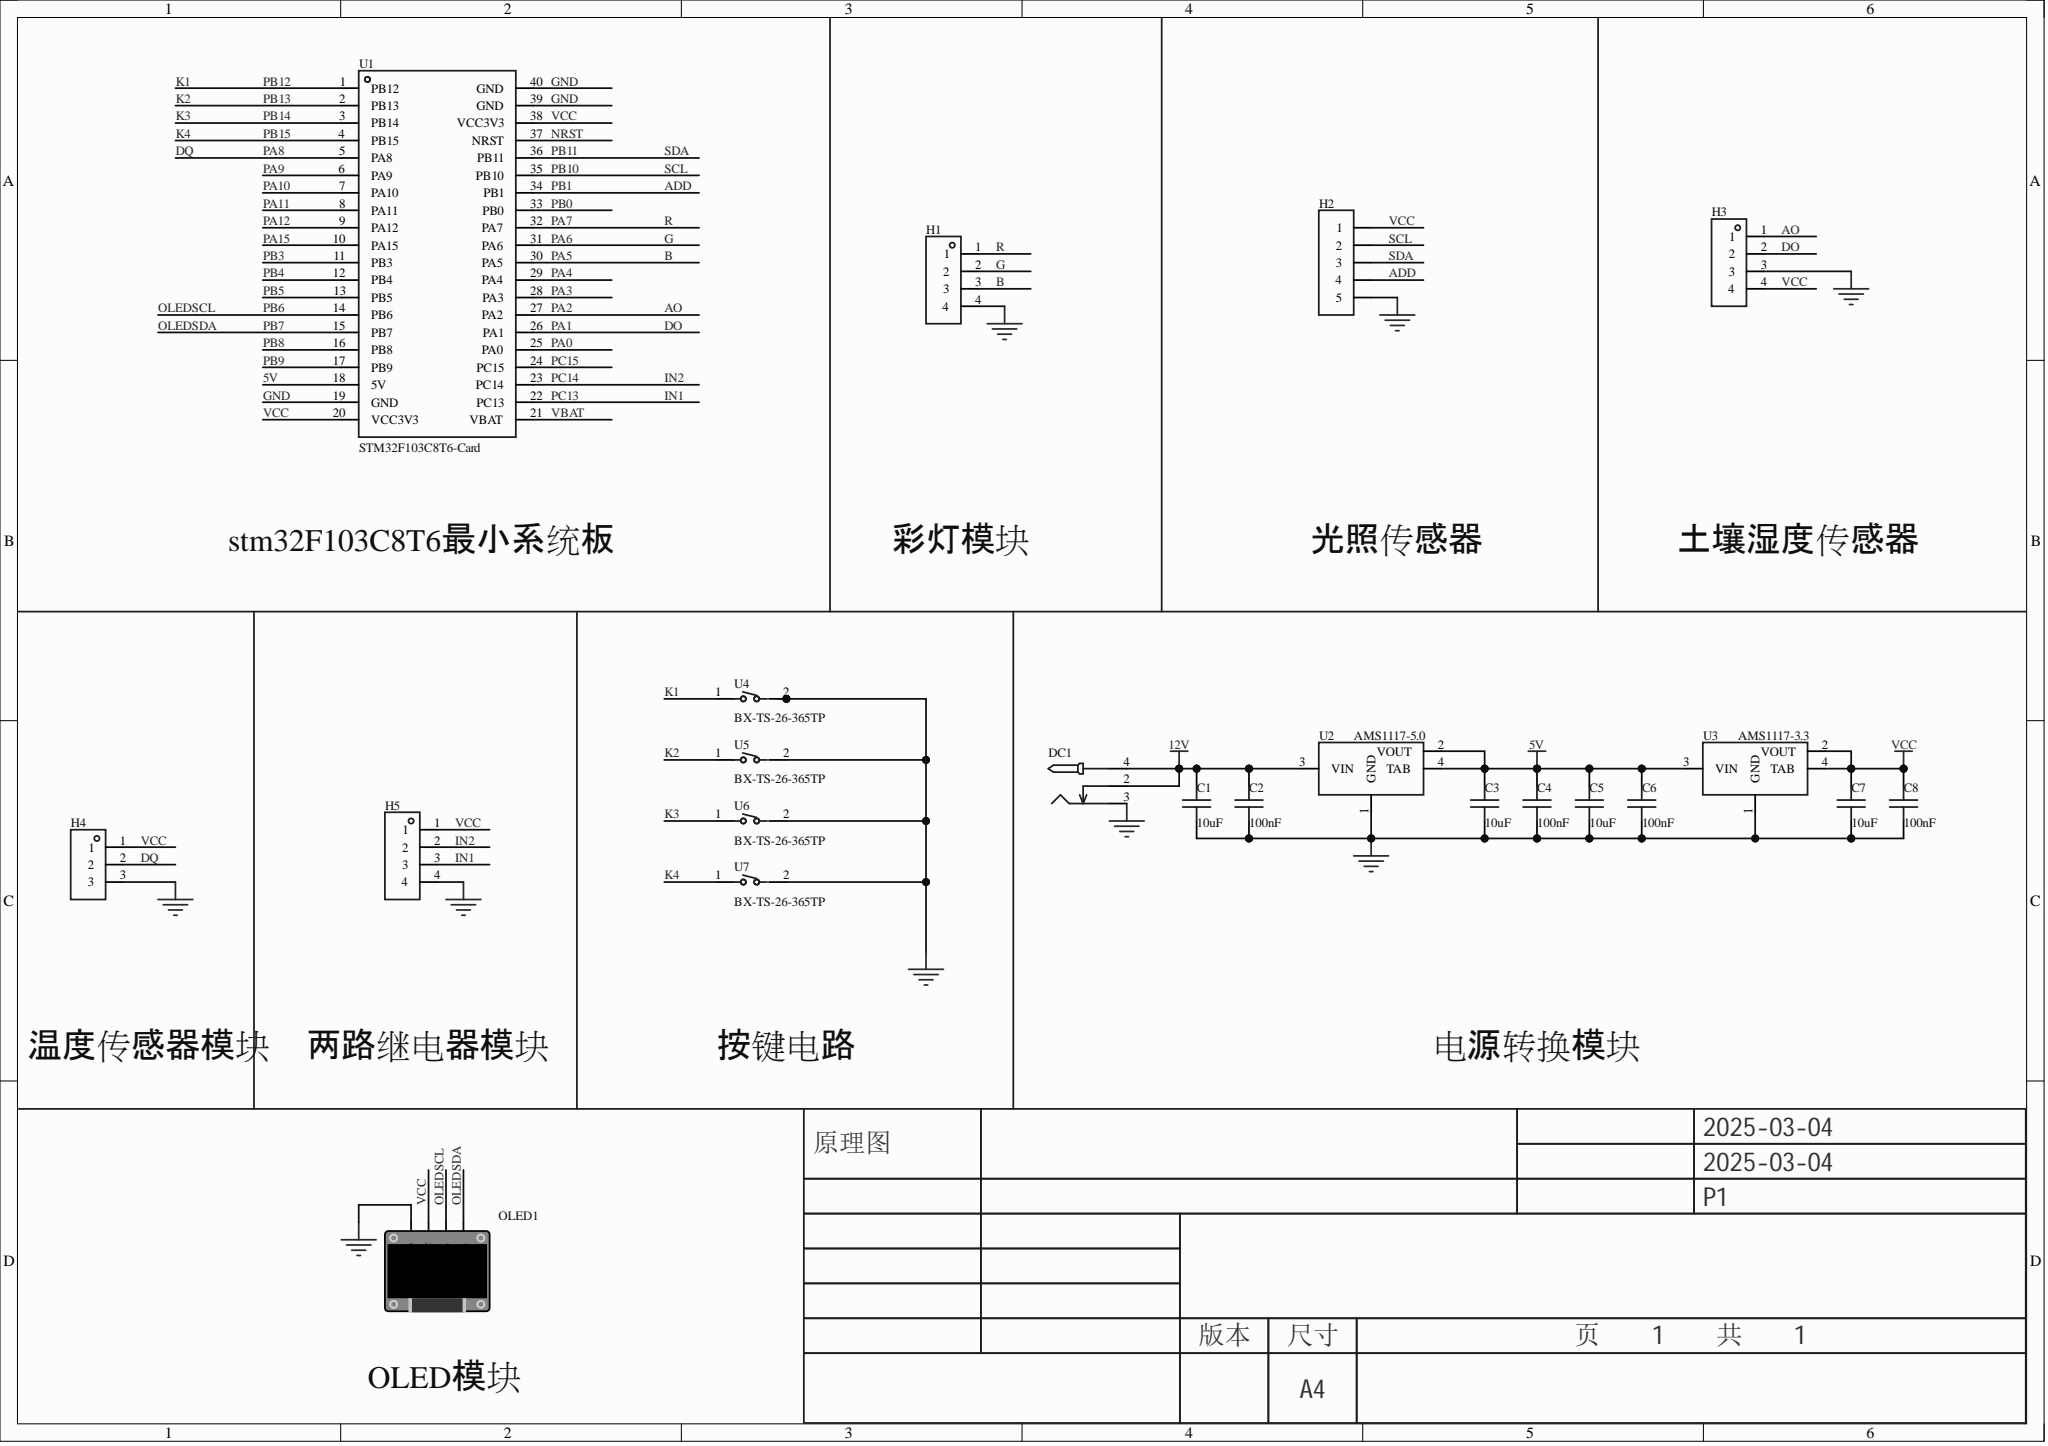Circuit board | Altium Designer | 22 parts | 21 nets
Bill of materials:
Comment,Description,Designator,Footprint,LibRef,Quantity
"10uF","","C1, C3, C5, C7","C0805","CAP_0805","4"
"100nF","","C2, C4, C6, C8","C0805","CAP_0805","4"
"","","DC1","DC-2.0","DC-005_2.0","1"
"","","H1, H3, H5","HDR-TH_4P-P2.54-V-F","HDR-F_2.54_1x4P","3"
"","","H2","HDR-TH_5P-P2.54-V-F","HDR-F_2.54_1x5P","1"
"","","H4","HDR-TH_3P-P2.54-V-F","HDR-F_2.54_1x3P","1"
"","","OLED1","0.96OLED_4P","0.96OLED模块_4P","1"
"STM32F103C8T6-Card","","U1","CONN-TH_L53.3-W22.9_STM32F103C8T6-CARD","STM32F103C8T6-Card","1"
"AMS1117-5.0","","U2","SOT_223","AMS1117","1"
"AMS1117-3.3","","U3","SOT_223","AMS1117","1"
"BX-TS-26-365TP","","U4, U5, U6, U7","KEY-SMD_L6.0-W3.5-LS8.0-1","BX-TS-26-365TP","4"
Netlist (Protel format):
[
C1
C0805
10uF



]
[
C2
C0805
100nF



]
[
C3
C0805
10uF



]
[
C4
C0805
100nF



]
[
C5
C0805
10uF



]
[
C6
C0805
100nF



]
[
C7
C0805
10uF



]
[
C8
C0805
100nF



]
[
DC1
DC-2.0




]
[
H1
HDR-TH_4P-P2.54-V-F




]
[
H2
HDR-TH_5P-P2.54-V-F




]
[
H3
HDR-TH_4P-P2.54-V-F




]
[
H4
HDR-TH_3P-P2.54-V-F




]
[
H5
HDR-TH_4P-P2.54-V-F




]
[
OLED1
0.96OLED_4P




]
[
U1
CONN-TH_L53.3-W22.9_STM32F103C8T6-CARD
STM32F103C8T6-Card



]
[
U2
SOT_223
AMS1117-5.0



]
[
U3
SOT_223
AMS1117-3.3



]
[
U4
KEY-SMD_L6.0-W3.5-LS8.0-1
BX-TS-26-365TP



]
[
U5
KEY-SMD_L6.0-W3.5-LS8.0-1
BX-TS-26-365TP



]
[
U6
KEY-SMD_L6.0-W3.5-LS8.0-1
BX-TS-26-365TP



]
[
U7
KEY-SMD_L6.0-W3.5-LS8.0-1
BX-TS-26-365TP



]
(
VCC
C7-2
C8-2
H2-1
H3-4
H4-1
H5-1
OLED1-2
U1-20
U1-38
U3-2
U3-4
)
(
PB11
H2-3
U1-36
)
(
PB10
H2-2
U1-35
)
(
PA7
H1-1
U1-32
)
(
OLEDSDA
OLED1-4
U1-15
)
(
OLEDSCL
OLED1-3
U1-14
)
(
K4
U1-4
U7-1
)
(
K3
U1-3
U6-1
)
(
K2
U1-2
U5-1
)
(
K1
U1-1
U4-1
)
(
IN2
H5-2
U1-23
)
(
IN1
H5-3
U1-22
)
(
GND
C1-1
C2-1
C3-1
C4-1
C5-1
C6-1
C7-1
C8-1
DC1-3
H1-4
H2-5
H3-3
H4-3
H5-4
OLED1-1
U1-19
U1-39
U1-40
U2-1
U3-1
U4-2
U5-2
U6-2
U7-2
)
(
G
H1-2
U1-31
)
(
DQ
H4-2
U1-5
)
(
DO
H3-2
U1-26
)
(
B
H1-3
U1-30
)
(
AO
H3-1
U1-27
)
(
ADD
H2-4
U1-34
)
(
12V
C1-2
C2-2
DC1-2
DC1-4
U2-3
)
(
5V
C3-2
C4-2
C5-2
C6-2
U1-18
U2-2
U2-4
U3-3
)